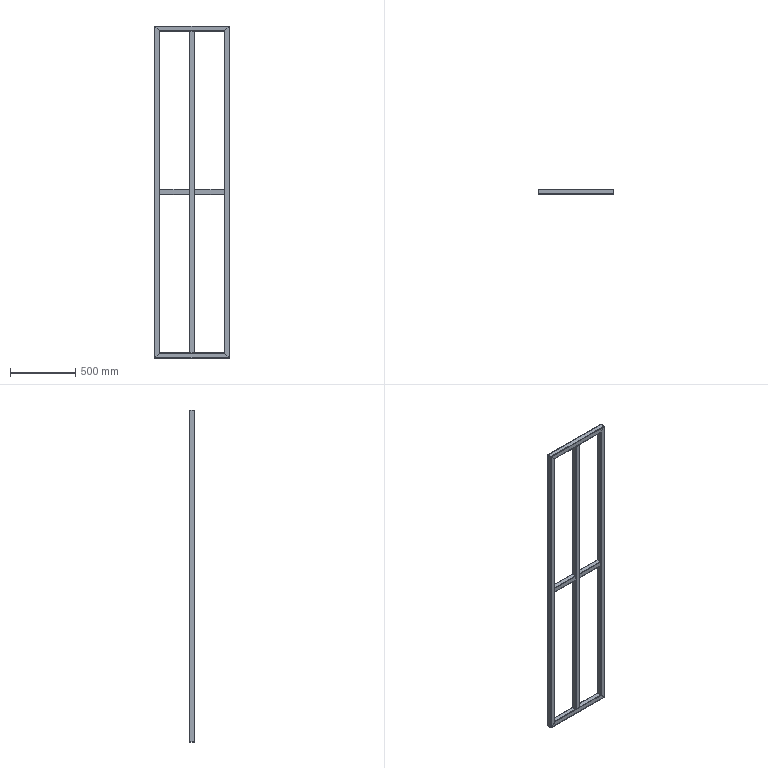Part | STEP file | Stopper rack_Default<Machined> | 7 solids | 126 faces | box 575 x 40 x 2540 mm | volume 2334872 mm3 | plane 70 | cylinder 56 | commonest cylinder face diameters 3.5 x28 7 x28